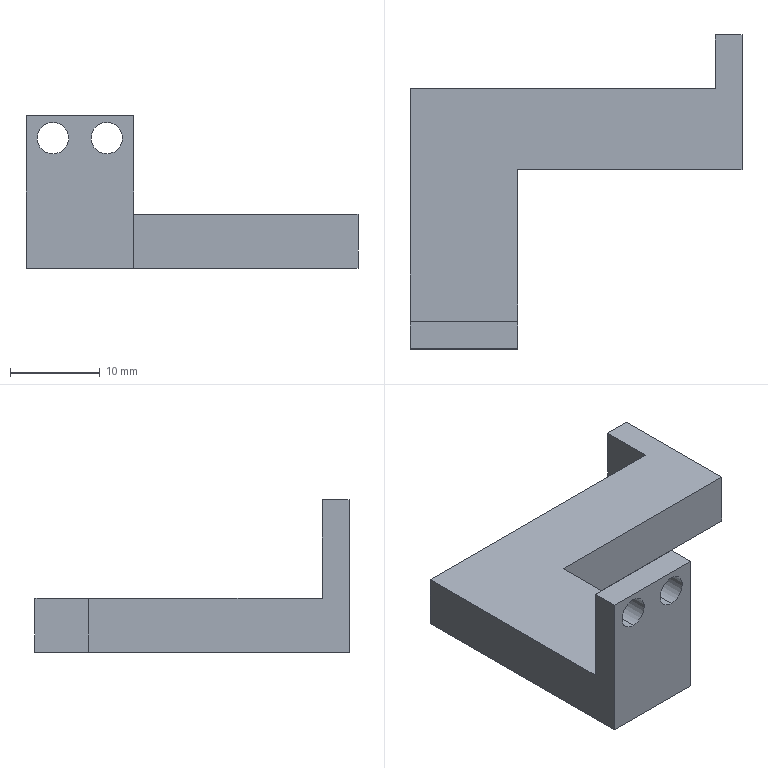Part | SolidWorks | features BaseBody 1 | 1 solid | 16 faces | box 37 x 35 x 17 mm | volume 3884 mm3 | plane 12 | cylinder 4 | commonest cylinder face diameters 3.5 x4
STEP:
#1=CARTESIAN_POINT('',(692.759,590.431,12.75));
#2=VERTEX_POINT('',#1);
#3=CARTESIAN_POINT('',(692.759,590.431,16.25));
#4=VERTEX_POINT('',#3);
#5=CARTESIAN_POINT('',(692.759,590.431,14.5));
#6=DIRECTION('',(0.,1.,0.));
#7=DIRECTION('',(0.,0.,1.));
#8=AXIS2_PLACEMENT_3D('',#5,#6,#7);
#9=CIRCLE('',#8,1.75);
#10=EDGE_CURVE('',#2,#4,#9,.T.);
#11=ORIENTED_EDGE('',*,*,#10,.F.);
#12=CARTESIAN_POINT('',(692.759,593.431,12.75));
#13=VERTEX_POINT('',#12);
#14=CARTESIAN_POINT('',(692.759,539.738,12.75));
#15=DIRECTION('',(0.,1.,0.));
#16=VECTOR('',#15,1000.);
#17=LINE('',#14,#16);
#18=EDGE_CURVE('',#2,#13,#17,.T.);
#19=ORIENTED_EDGE('',*,*,#18,.T.);
#20=CARTESIAN_POINT('',(692.759,593.431,16.25));
#21=VERTEX_POINT('',#20);
#22=CARTESIAN_POINT('',(692.759,593.431,14.5));
#23=DIRECTION('',(0.,1.,0.));
#24=DIRECTION('',(0.,0.,1.));
#25=AXIS2_PLACEMENT_3D('',#22,#23,#24);
#26=CIRCLE('',#25,1.75);
#27=EDGE_CURVE('',#13,#21,#26,.T.);
#28=ORIENTED_EDGE('',*,*,#27,.T.);
#29=CARTESIAN_POINT('',(692.759,539.738,16.25));
#30=DIRECTION('',(0.,1.,0.));
#31=VECTOR('',#30,1000.);
#32=LINE('',#29,#31);
#33=EDGE_CURVE('',#4,#21,#32,.T.);
#34=ORIENTED_EDGE('',*,*,#33,.F.);
#35=EDGE_LOOP('',(#11,#19,#28,#34));
#36=FACE_OUTER_BOUND('',#35,.T.);
#37=CARTESIAN_POINT('',(692.759,539.738,14.5));
#38=DIRECTION('',(0.,1.,0.));
#39=DIRECTION('',(0.,0.,1.));
#40=AXIS2_PLACEMENT_3D('',#37,#38,#39);
#41=CYLINDRICAL_SURFACE('',#40,1.75);
#42=ADVANCED_FACE('',(#36),#41,.F.);
#43=CARTESIAN_POINT('',(698.759,590.431,12.75));
#44=VERTEX_POINT('',#43);
#45=CARTESIAN_POINT('',(698.759,590.431,16.25));
#46=VERTEX_POINT('',#45);
#47=CARTESIAN_POINT('',(698.759,590.431,14.5));
#48=DIRECTION('',(0.,1.,0.));
#49=DIRECTION('',(0.,0.,1.));
#50=AXIS2_PLACEMENT_3D('',#47,#48,#49);
#51=CIRCLE('',#50,1.75);
#52=EDGE_CURVE('',#44,#46,#51,.T.);
#53=ORIENTED_EDGE('',*,*,#52,.F.);
#54=CARTESIAN_POINT('',(698.759,593.431,12.75));
#55=VERTEX_POINT('',#54);
#56=CARTESIAN_POINT('',(698.759,539.738,12.75));
#57=DIRECTION('',(0.,1.,0.));
#58=VECTOR('',#57,1000.);
#59=LINE('',#56,#58);
#60=EDGE_CURVE('',#44,#55,#59,.T.);
#61=ORIENTED_EDGE('',*,*,#60,.T.);
#62=CARTESIAN_POINT('',(698.759,593.431,16.25));
#63=VERTEX_POINT('',#62);
#64=CARTESIAN_POINT('',(698.759,593.431,14.5));
#65=DIRECTION('',(0.,1.,0.));
#66=DIRECTION('',(0.,0.,1.));
#67=AXIS2_PLACEMENT_3D('',#64,#65,#66);
#68=CIRCLE('',#67,1.75);
#69=EDGE_CURVE('',#55,#63,#68,.T.);
#70=ORIENTED_EDGE('',*,*,#69,.T.);
#71=CARTESIAN_POINT('',(698.759,539.738,16.25));
#72=DIRECTION('',(0.,1.,0.));
#73=VECTOR('',#72,1000.);
#74=LINE('',#71,#73);
#75=EDGE_CURVE('',#46,#63,#74,.T.);
#76=ORIENTED_EDGE('',*,*,#75,.F.);
#77=EDGE_LOOP('',(#53,#61,#70,#76));
#78=FACE_OUTER_BOUND('',#77,.T.);
#79=CARTESIAN_POINT('',(698.759,539.738,14.5));
#80=DIRECTION('',(0.,1.,0.));
#81=DIRECTION('',(0.,0.,1.));
#82=AXIS2_PLACEMENT_3D('',#79,#80,#81);
#83=CYLINDRICAL_SURFACE('',#82,1.75);
#84=ADVANCED_FACE('',(#78),#83,.F.);
#85=CARTESIAN_POINT('',(701.759,590.431,0.));
#86=VERTEX_POINT('',#85);
#87=CARTESIAN_POINT('',(701.759,610.431,0.));
#88=VERTEX_POINT('',#87);
#89=CARTESIAN_POINT('',(701.759,607.931,0.));
#90=DIRECTION('',(0.,1.,0.));
#91=VECTOR('',#90,1000.);
#92=LINE('',#89,#91);
#93=EDGE_CURVE('',#86,#88,#92,.T.);
#94=ORIENTED_EDGE('',*,*,#93,.F.);
#95=CARTESIAN_POINT('',(689.759,590.431,0.));
#96=VERTEX_POINT('',#95);
#97=CARTESIAN_POINT('',(708.259,590.431,0.));
#98=DIRECTION('',(1.,0.,0.));
#99=VECTOR('',#98,1000.);
#100=LINE('',#97,#99);
#101=EDGE_CURVE('',#96,#86,#100,.T.);
#102=ORIENTED_EDGE('',*,*,#101,.F.);
#103=CARTESIAN_POINT('',(689.759,619.431,0.));
#104=VERTEX_POINT('',#103);
#105=CARTESIAN_POINT('',(689.759,607.931,0.));
#106=DIRECTION('',(0.,-1.,0.));
#107=VECTOR('',#106,1000.);
#108=LINE('',#105,#107);
#109=EDGE_CURVE('',#104,#96,#108,.T.);
#110=ORIENTED_EDGE('',*,*,#109,.F.);
#111=CARTESIAN_POINT('',(723.759,619.431,0.));
#112=VERTEX_POINT('',#111);
#113=CARTESIAN_POINT('',(708.259,619.431,0.));
#114=DIRECTION('',(-1.,0.,0.));
#115=VECTOR('',#114,1000.);
#116=LINE('',#113,#115);
#117=EDGE_CURVE('',#112,#104,#116,.T.);
#118=ORIENTED_EDGE('',*,*,#117,.F.);
#119=CARTESIAN_POINT('',(723.759,625.431,0.));
#120=VERTEX_POINT('',#119);
#121=CARTESIAN_POINT('',(723.759,607.931,0.));
#122=DIRECTION('',(0.,-1.,0.));
#123=VECTOR('',#122,1000.);
#124=LINE('',#121,#123);
#125=EDGE_CURVE('',#120,#112,#124,.T.);
#126=ORIENTED_EDGE('',*,*,#125,.F.);
#127=CARTESIAN_POINT('',(726.759,625.431,0.));
#128=VERTEX_POINT('',#127);
#129=CARTESIAN_POINT('',(708.259,625.431,0.));
#130=DIRECTION('',(-1.,0.,0.));
#131=VECTOR('',#130,1000.);
#132=LINE('',#129,#131);
#133=EDGE_CURVE('',#128,#120,#132,.T.);
#134=ORIENTED_EDGE('',*,*,#133,.F.);
#135=CARTESIAN_POINT('',(726.759,610.431,0.));
#136=VERTEX_POINT('',#135);
#137=CARTESIAN_POINT('',(726.759,607.931,0.));
#138=DIRECTION('',(0.,1.,0.));
#139=VECTOR('',#138,1000.);
#140=LINE('',#137,#139);
#141=EDGE_CURVE('',#136,#128,#140,.T.);
#142=ORIENTED_EDGE('',*,*,#141,.F.);
#143=CARTESIAN_POINT('',(708.259,610.431,0.));
#144=DIRECTION('',(1.,0.,0.));
#145=VECTOR('',#144,1000.);
#146=LINE('',#143,#145);
#147=EDGE_CURVE('',#88,#136,#146,.T.);
#148=ORIENTED_EDGE('',*,*,#147,.F.);
#149=EDGE_LOOP('',(#94,#102,#110,#118,#126,#134,#142,#148));
#150=FACE_OUTER_BOUND('',#149,.T.);
#151=CARTESIAN_POINT('',(708.259,607.931,0.));
#152=DIRECTION('',(0.,0.,1.));
#153=DIRECTION('',(1.,0.,0.));
#154=AXIS2_PLACEMENT_3D('',#151,#152,#153);
#155=PLANE('',#154);
#156=ADVANCED_FACE('',(#150),#155,.F.);
#157=CARTESIAN_POINT('',(726.759,610.431,6.));
#158=VERTEX_POINT('',#157);
#159=CARTESIAN_POINT('',(726.759,610.431,6.));
#160=DIRECTION('',(0.,0.,-1.));
#161=VECTOR('',#160,1000.);
#162=LINE('',#159,#161);
#163=EDGE_CURVE('',#158,#136,#162,.T.);
#164=ORIENTED_EDGE('',*,*,#163,.F.);
#165=CARTESIAN_POINT('',(701.759,610.431,6.));
#166=VERTEX_POINT('',#165);
#167=CARTESIAN_POINT('',(726.759,610.431,6.));
#168=DIRECTION('',(1.,0.,0.));
#169=VECTOR('',#168,1000.);
#170=LINE('',#167,#169);
#171=EDGE_CURVE('',#166,#158,#170,.T.);
#172=ORIENTED_EDGE('',*,*,#171,.F.);
#173=CARTESIAN_POINT('',(701.759,610.431,6.));
#174=DIRECTION('',(0.,0.,1.));
#175=VECTOR('',#174,1000.);
#176=LINE('',#173,#175);
#177=EDGE_CURVE('',#88,#166,#176,.T.);
#178=ORIENTED_EDGE('',*,*,#177,.F.);
#179=ORIENTED_EDGE('',*,*,#147,.T.);
#180=EDGE_LOOP('',(#164,#172,#178,#179));
#181=FACE_OUTER_BOUND('',#180,.T.);
#182=CARTESIAN_POINT('',(726.759,610.431,6.));
#183=DIRECTION('',(0.,1.,0.));
#184=DIRECTION('',(0.,0.,1.));
#185=AXIS2_PLACEMENT_3D('',#182,#183,#184);
#186=PLANE('',#185);
#187=ADVANCED_FACE('',(#181),#186,.F.);
#188=CARTESIAN_POINT('',(701.759,590.431,17.));
#189=VERTEX_POINT('',#188);
#190=CARTESIAN_POINT('',(701.759,593.431,17.));
#191=VERTEX_POINT('',#190);
#192=CARTESIAN_POINT('',(701.759,593.431,17.));
#193=DIRECTION('',(0.,1.,0.));
#194=VECTOR('',#193,1000.);
#195=LINE('',#192,#194);
#196=EDGE_CURVE('',#189,#191,#195,.T.);
#197=ORIENTED_EDGE('',*,*,#196,.F.);
#198=CARTESIAN_POINT('',(701.759,590.431,17.));
#199=DIRECTION('',(0.,0.,1.));
#200=VECTOR('',#199,1000.);
#201=LINE('',#198,#200);
#202=EDGE_CURVE('',#86,#189,#201,.T.);
#203=ORIENTED_EDGE('',*,*,#202,.F.);
#204=ORIENTED_EDGE('',*,*,#93,.T.);
#205=ORIENTED_EDGE('',*,*,#177,.T.);
#206=CARTESIAN_POINT('',(701.759,593.431,6.));
#207=VERTEX_POINT('',#206);
#208=CARTESIAN_POINT('',(701.759,593.431,6.));
#209=DIRECTION('',(0.,1.,0.));
#210=VECTOR('',#209,1000.);
#211=LINE('',#208,#210);
#212=EDGE_CURVE('',#207,#166,#211,.T.);
#213=ORIENTED_EDGE('',*,*,#212,.F.);
#214=CARTESIAN_POINT('',(701.759,593.431,17.));
#215=DIRECTION('',(0.,0.,-1.));
#216=VECTOR('',#215,1000.);
#217=LINE('',#214,#216);
#218=EDGE_CURVE('',#191,#207,#217,.T.);
#219=ORIENTED_EDGE('',*,*,#218,.F.);
#220=EDGE_LOOP('',(#197,#203,#204,#205,#213,#219));
#221=FACE_OUTER_BOUND('',#220,.T.);
#222=CARTESIAN_POINT('',(701.759,593.431,17.));
#223=DIRECTION('',(-1.,0.,0.));
#224=DIRECTION('',(0.,0.,1.));
#225=AXIS2_PLACEMENT_3D('',#222,#223,#224);
#226=PLANE('',#225);
#227=ADVANCED_FACE('',(#221),#226,.F.);
#228=CARTESIAN_POINT('',(692.759,590.431,14.5));
#229=DIRECTION('',(0.,1.,0.));
#230=DIRECTION('',(0.,0.,1.));
#231=AXIS2_PLACEMENT_3D('',#228,#229,#230);
#232=CIRCLE('',#231,1.75);
#233=EDGE_CURVE('',#4,#2,#232,.T.);
#234=ORIENTED_EDGE('',*,*,#233,.T.);
#235=ORIENTED_EDGE('',*,*,#10,.T.);
#236=EDGE_LOOP('',(#234,#235));
#237=FACE_BOUND('',#236,.T.);
#238=CARTESIAN_POINT('',(698.759,590.431,14.5));
#239=DIRECTION('',(0.,1.,0.));
#240=DIRECTION('',(0.,0.,1.));
#241=AXIS2_PLACEMENT_3D('',#238,#239,#240);
#242=CIRCLE('',#241,1.75);
#243=EDGE_CURVE('',#46,#44,#242,.T.);
#244=ORIENTED_EDGE('',*,*,#243,.T.);
#245=ORIENTED_EDGE('',*,*,#52,.T.);
#246=EDGE_LOOP('',(#244,#245));
#247=FACE_BOUND('',#246,.T.);
#248=CARTESIAN_POINT('',(689.759,590.431,17.));
#249=VERTEX_POINT('',#248);
#250=CARTESIAN_POINT('',(689.759,590.431,0.));
#251=DIRECTION('',(0.,0.,-1.));
#252=VECTOR('',#251,1000.);
#253=LINE('',#250,#252);
#254=EDGE_CURVE('',#249,#96,#253,.T.);
#255=ORIENTED_EDGE('',*,*,#254,.T.);
#256=ORIENTED_EDGE('',*,*,#101,.T.);
#257=ORIENTED_EDGE('',*,*,#202,.T.);
#258=CARTESIAN_POINT('',(726.759,590.431,17.));
#259=DIRECTION('',(-1.,0.,0.));
#260=VECTOR('',#259,1000.);
#261=LINE('',#258,#260);
#262=EDGE_CURVE('',#189,#249,#261,.T.);
#263=ORIENTED_EDGE('',*,*,#262,.T.);
#264=EDGE_LOOP('',(#255,#256,#257,#263));
#265=FACE_OUTER_BOUND('',#264,.T.);
#266=CARTESIAN_POINT('',(726.759,590.431,0.));
#267=DIRECTION('',(0.,-1.,0.));
#268=DIRECTION('',(0.,0.,-1.));
#269=AXIS2_PLACEMENT_3D('',#266,#267,#268);
#270=PLANE('',#269);
#271=ADVANCED_FACE('',(#237,#247,#265),#270,.T.);
#272=CARTESIAN_POINT('',(689.759,593.431,17.));
#273=VERTEX_POINT('',#272);
#274=CARTESIAN_POINT('',(689.759,593.431,6.));
#275=VERTEX_POINT('',#274);
#276=CARTESIAN_POINT('',(689.759,593.431,0.));
#277=DIRECTION('',(0.,0.,-1.));
#278=VECTOR('',#277,1000.);
#279=LINE('',#276,#278);
#280=EDGE_CURVE('',#273,#275,#279,.T.);
#281=ORIENTED_EDGE('',*,*,#280,.T.);
#282=CARTESIAN_POINT('',(689.759,619.431,6.));
#283=VERTEX_POINT('',#282);
#284=CARTESIAN_POINT('',(689.759,590.431,6.));
#285=DIRECTION('',(0.,1.,0.));
#286=VECTOR('',#285,1000.);
#287=LINE('',#284,#286);
#288=EDGE_CURVE('',#275,#283,#287,.T.);
#289=ORIENTED_EDGE('',*,*,#288,.T.);
#290=CARTESIAN_POINT('',(689.759,619.431,0.));
#291=DIRECTION('',(0.,0.,-1.));
#292=VECTOR('',#291,1000.);
#293=LINE('',#290,#292);
#294=EDGE_CURVE('',#283,#104,#293,.T.);
#295=ORIENTED_EDGE('',*,*,#294,.T.);
#296=ORIENTED_EDGE('',*,*,#109,.T.);
#297=ORIENTED_EDGE('',*,*,#254,.F.);
#298=CARTESIAN_POINT('',(689.759,590.431,17.));
#299=DIRECTION('',(0.,1.,0.));
#300=VECTOR('',#299,1000.);
#301=LINE('',#298,#300);
#302=EDGE_CURVE('',#249,#273,#301,.T.);
#303=ORIENTED_EDGE('',*,*,#302,.T.);
#304=EDGE_LOOP('',(#281,#289,#295,#296,#297,#303));
#305=FACE_OUTER_BOUND('',#304,.T.);
#306=CARTESIAN_POINT('',(689.759,590.431,0.));
#307=DIRECTION('',(-1.,0.,0.));
#308=DIRECTION('',(0.,0.,1.));
#309=AXIS2_PLACEMENT_3D('',#306,#307,#308);
#310=PLANE('',#309);
#311=ADVANCED_FACE('',(#305),#310,.T.);
#312=ORIENTED_EDGE('',*,*,#294,.F.);
#313=CARTESIAN_POINT('',(723.759,619.431,6.));
#314=VERTEX_POINT('',#313);
#315=CARTESIAN_POINT('',(689.759,619.431,6.));
#316=DIRECTION('',(-1.,0.,0.));
#317=VECTOR('',#316,1000.);
#318=LINE('',#315,#317);
#319=EDGE_CURVE('',#314,#283,#318,.T.);
#320=ORIENTED_EDGE('',*,*,#319,.F.);
#321=CARTESIAN_POINT('',(723.759,619.431,6.));
#322=DIRECTION('',(0.,0.,1.));
#323=VECTOR('',#322,1000.);
#324=LINE('',#321,#323);
#325=EDGE_CURVE('',#112,#314,#324,.T.);
#326=ORIENTED_EDGE('',*,*,#325,.F.);
#327=ORIENTED_EDGE('',*,*,#117,.T.);
#328=EDGE_LOOP('',(#312,#320,#326,#327));
#329=FACE_OUTER_BOUND('',#328,.T.);
#330=CARTESIAN_POINT('',(689.759,619.431,6.));
#331=DIRECTION('',(0.,-1.,0.));
#332=DIRECTION('',(0.,0.,-1.));
#333=AXIS2_PLACEMENT_3D('',#330,#331,#332);
#334=PLANE('',#333);
#335=ADVANCED_FACE('',(#329),#334,.F.);
#336=ORIENTED_EDGE('',*,*,#325,.T.);
#337=CARTESIAN_POINT('',(723.759,625.431,6.));
#338=VERTEX_POINT('',#337);
#339=CARTESIAN_POINT('',(723.759,619.431,6.));
#340=DIRECTION('',(0.,-1.,0.));
#341=VECTOR('',#340,1000.);
#342=LINE('',#339,#341);
#343=EDGE_CURVE('',#338,#314,#342,.T.);
#344=ORIENTED_EDGE('',*,*,#343,.F.);
#345=CARTESIAN_POINT('',(723.759,625.431,6.));
#346=DIRECTION('',(0.,0.,1.));
#347=VECTOR('',#346,1000.);
#348=LINE('',#345,#347);
#349=EDGE_CURVE('',#120,#338,#348,.T.);
#350=ORIENTED_EDGE('',*,*,#349,.F.);
#351=ORIENTED_EDGE('',*,*,#125,.T.);
#352=EDGE_LOOP('',(#336,#344,#350,#351));
#353=FACE_OUTER_BOUND('',#352,.T.);
#354=CARTESIAN_POINT('',(723.759,619.431,6.));
#355=DIRECTION('',(1.,0.,0.));
#356=DIRECTION('',(0.,0.,-1.));
#357=AXIS2_PLACEMENT_3D('',#354,#355,#356);
#358=PLANE('',#357);
#359=ADVANCED_FACE('',(#353),#358,.F.);
#360=CARTESIAN_POINT('',(726.759,625.431,6.));
#361=VERTEX_POINT('',#360);
#362=CARTESIAN_POINT('',(726.759,625.431,0.));
#363=DIRECTION('',(0.,0.,-1.));
#364=VECTOR('',#363,1000.);
#365=LINE('',#362,#364);
#366=EDGE_CURVE('',#361,#128,#365,.T.);
#367=ORIENTED_EDGE('',*,*,#366,.T.);
#368=ORIENTED_EDGE('',*,*,#133,.T.);
#369=ORIENTED_EDGE('',*,*,#349,.T.);
#370=CARTESIAN_POINT('',(689.759,625.431,6.));
#371=DIRECTION('',(1.,0.,0.));
#372=VECTOR('',#371,1000.);
#373=LINE('',#370,#372);
#374=EDGE_CURVE('',#338,#361,#373,.T.);
#375=ORIENTED_EDGE('',*,*,#374,.T.);
#376=EDGE_LOOP('',(#367,#368,#369,#375));
#377=FACE_OUTER_BOUND('',#376,.T.);
#378=CARTESIAN_POINT('',(689.759,625.431,0.));
#379=DIRECTION('',(0.,1.,0.));
#380=DIRECTION('',(0.,0.,1.));
#381=AXIS2_PLACEMENT_3D('',#378,#379,#380);
#382=PLANE('',#381);
#383=ADVANCED_FACE('',(#377),#382,.T.);
#384=ORIENTED_EDGE('',*,*,#366,.F.);
#385=CARTESIAN_POINT('',(726.759,625.431,6.));
#386=DIRECTION('',(0.,-1.,0.));
#387=VECTOR('',#386,1000.);
#388=LINE('',#385,#387);
#389=EDGE_CURVE('',#361,#158,#388,.T.);
#390=ORIENTED_EDGE('',*,*,#389,.T.);
#391=ORIENTED_EDGE('',*,*,#163,.T.);
#392=ORIENTED_EDGE('',*,*,#141,.T.);
#393=EDGE_LOOP('',(#384,#390,#391,#392));
#394=FACE_OUTER_BOUND('',#393,.T.);
#395=CARTESIAN_POINT('',(726.759,625.431,0.));
#396=DIRECTION('',(1.,0.,0.));
#397=DIRECTION('',(0.,0.,-1.));
#398=AXIS2_PLACEMENT_3D('',#395,#396,#397);
#399=PLANE('',#398);
#400=ADVANCED_FACE('',(#394),#399,.T.);
#401=CARTESIAN_POINT('',(708.509,593.431,6.));
#402=DIRECTION('',(1.,0.,0.));
#403=VECTOR('',#402,1000.);
#404=LINE('',#401,#403);
#405=EDGE_CURVE('',#275,#207,#404,.T.);
#406=ORIENTED_EDGE('',*,*,#405,.T.);
#407=ORIENTED_EDGE('',*,*,#212,.T.);
#408=ORIENTED_EDGE('',*,*,#171,.T.);
#409=ORIENTED_EDGE('',*,*,#389,.F.);
#410=ORIENTED_EDGE('',*,*,#374,.F.);
#411=ORIENTED_EDGE('',*,*,#343,.T.);
#412=ORIENTED_EDGE('',*,*,#319,.T.);
#413=ORIENTED_EDGE('',*,*,#288,.F.);
#414=EDGE_LOOP('',(#406,#407,#408,#409,#410,#411,#412,#413));
#415=FACE_OUTER_BOUND('',#414,.T.);
#416=CARTESIAN_POINT('',(708.509,608.181,6.));
#417=DIRECTION('',(0.,0.,1.));
#418=DIRECTION('',(1.,0.,0.));
#419=AXIS2_PLACEMENT_3D('',#416,#417,#418);
#420=PLANE('',#419);
#421=ADVANCED_FACE('',(#415),#420,.T.);
#422=CARTESIAN_POINT('',(692.759,593.431,14.5));
#423=DIRECTION('',(0.,1.,0.));
#424=DIRECTION('',(0.,0.,1.));
#425=AXIS2_PLACEMENT_3D('',#422,#423,#424);
#426=CIRCLE('',#425,1.75);
#427=EDGE_CURVE('',#21,#13,#426,.T.);
#428=ORIENTED_EDGE('',*,*,#427,.F.);
#429=ORIENTED_EDGE('',*,*,#27,.F.);
#430=EDGE_LOOP('',(#428,#429));
#431=FACE_BOUND('',#430,.T.);
#432=CARTESIAN_POINT('',(698.759,593.431,14.5));
#433=DIRECTION('',(0.,1.,0.));
#434=DIRECTION('',(0.,0.,1.));
#435=AXIS2_PLACEMENT_3D('',#432,#433,#434);
#436=CIRCLE('',#435,1.75);
#437=EDGE_CURVE('',#63,#55,#436,.T.);
#438=ORIENTED_EDGE('',*,*,#437,.F.);
#439=ORIENTED_EDGE('',*,*,#69,.F.);
#440=EDGE_LOOP('',(#438,#439));
#441=FACE_BOUND('',#440,.T.);
#442=ORIENTED_EDGE('',*,*,#280,.F.);
#443=CARTESIAN_POINT('',(689.759,593.431,17.));
#444=DIRECTION('',(-1.,0.,0.));
#445=VECTOR('',#444,1000.);
#446=LINE('',#443,#445);
#447=EDGE_CURVE('',#191,#273,#446,.T.);
#448=ORIENTED_EDGE('',*,*,#447,.F.);
#449=ORIENTED_EDGE('',*,*,#218,.T.);
#450=ORIENTED_EDGE('',*,*,#405,.F.);
#451=EDGE_LOOP('',(#442,#448,#449,#450));
#452=FACE_OUTER_BOUND('',#451,.T.);
#453=CARTESIAN_POINT('',(689.759,593.431,17.));
#454=DIRECTION('',(0.,-1.,0.));
#455=DIRECTION('',(0.,0.,-1.));
#456=AXIS2_PLACEMENT_3D('',#453,#454,#455);
#457=PLANE('',#456);
#458=ADVANCED_FACE('',(#431,#441,#452),#457,.F.);
#459=ORIENTED_EDGE('',*,*,#302,.F.);
#460=ORIENTED_EDGE('',*,*,#262,.F.);
#461=ORIENTED_EDGE('',*,*,#196,.T.);
#462=ORIENTED_EDGE('',*,*,#447,.T.);
#463=EDGE_LOOP('',(#459,#460,#461,#462));
#464=FACE_OUTER_BOUND('',#463,.T.);
#465=CARTESIAN_POINT('',(708.259,607.931,17.));
#466=DIRECTION('',(0.,0.,1.));
#467=DIRECTION('',(1.,0.,0.));
#468=AXIS2_PLACEMENT_3D('',#465,#466,#467);
#469=PLANE('',#468);
#470=ADVANCED_FACE('',(#464),#469,.T.);
#471=ORIENTED_EDGE('',*,*,#18,.F.);
#472=ORIENTED_EDGE('',*,*,#233,.F.);
#473=ORIENTED_EDGE('',*,*,#33,.T.);
#474=ORIENTED_EDGE('',*,*,#427,.T.);
#475=EDGE_LOOP('',(#471,#472,#473,#474));
#476=FACE_OUTER_BOUND('',#475,.T.);
#477=CARTESIAN_POINT('',(692.759,539.738,14.5));
#478=DIRECTION('',(0.,1.,0.));
#479=DIRECTION('',(0.,0.,1.));
#480=AXIS2_PLACEMENT_3D('',#477,#478,#479);
#481=CYLINDRICAL_SURFACE('',#480,1.75);
#482=ADVANCED_FACE('',(#476),#481,.F.);
#483=ORIENTED_EDGE('',*,*,#60,.F.);
#484=ORIENTED_EDGE('',*,*,#243,.F.);
#485=ORIENTED_EDGE('',*,*,#75,.T.);
#486=ORIENTED_EDGE('',*,*,#437,.T.);
#487=EDGE_LOOP('',(#483,#484,#485,#486));
#488=FACE_OUTER_BOUND('',#487,.T.);
#489=CARTESIAN_POINT('',(698.759,539.738,14.5));
#490=DIRECTION('',(0.,1.,0.));
#491=DIRECTION('',(0.,0.,1.));
#492=AXIS2_PLACEMENT_3D('',#489,#490,#491);
#493=CYLINDRICAL_SURFACE('',#492,1.75);
#494=ADVANCED_FACE('',(#488),#493,.F.);
#495=CLOSED_SHELL('',(#42,#84,#156,#187,#227,#271,#311,#335,#359,#383,#400,#421,#458,#470,#482,#494));
#496=MANIFOLD_SOLID_BREP('',#495);
#497=CARTESIAN_POINT('',(0.,0.,0.));
#498=DIRECTION('',(0.,0.,1.));
#499=DIRECTION('',(1.,0.,0.));
#500=AXIS2_PLACEMENT_3D('',#497,#498,#499);
#501=(LENGTH_UNIT()NAMED_UNIT(*)SI_UNIT(.MILLI.,.METRE.));
#502=UNCERTAINTY_MEASURE_WITH_UNIT(LENGTH_MEASURE(0.00001),#501,'','');
#503=(NAMED_UNIT(*)PLANE_ANGLE_UNIT()SI_UNIT($,.RADIAN.));
#504=(NAMED_UNIT(*)SI_UNIT($,.STERADIAN.)SOLID_ANGLE_UNIT());
#505=(GEOMETRIC_REPRESENTATION_CONTEXT(3)GLOBAL_UNCERTAINTY_ASSIGNED_CONTEXT((#502))GLOBAL_UNIT_ASSIGNED_CONTEXT((#501,#503,#504))REPRESENTATION_CONTEXT('',''));
#506=ADVANCED_BREP_SHAPE_REPRESENTATION('',(#496,#500),#505);